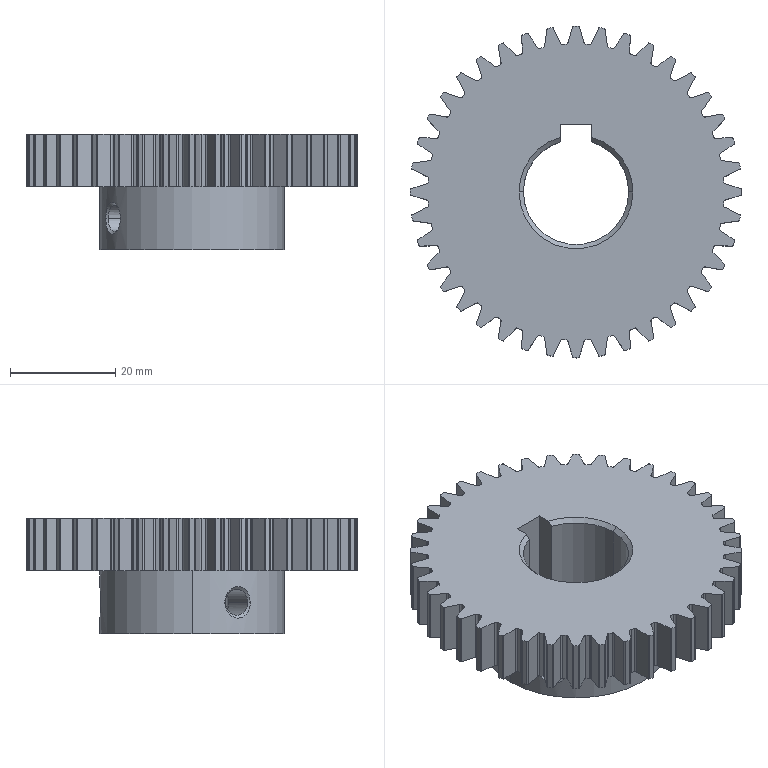Part | NX | features BREP 1 | 1 solid | 380 faces | box 63 x 63 x 22 mm | volume 31779 mm3 | cylinder 284 | plane 86 | cone 10 | commonest cylinder face diameters 0.75 x98 0.4 x96 63 x41 56.25 x40 4.917 x4 20 x3